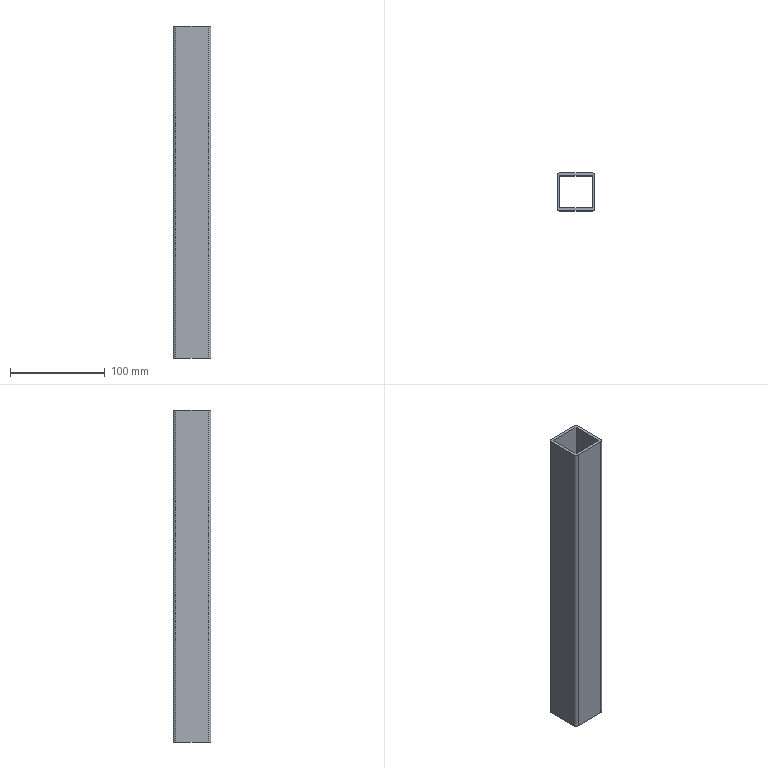Part | STEP file | X77-03114 | 1 solid | 14 faces | box 40 x 40 x 350 mm | volume 152696 mm3 | plane 10 | cylinder 4 | commonest cylinder face diameters 6 x4
STEP:
#1=CARTESIAN_POINT('',(-20.,-17.,350.));
#2=VERTEX_POINT('',#1);
#3=CARTESIAN_POINT('',(-17.,-20.,350.));
#4=VERTEX_POINT('',#3);
#5=CARTESIAN_POINT('',(-17.,-17.,350.));
#6=DIRECTION('',(0.,0.,1.));
#7=DIRECTION('',(-1.,0.,0.));
#8=AXIS2_PLACEMENT_3D('',#5,#6,#7);
#9=CIRCLE('',#8,3.);
#10=EDGE_CURVE('',#2,#4,#9,.T.);
#11=ORIENTED_EDGE('',*,*,#10,.T.);
#12=CARTESIAN_POINT('',(17.,-20.,350.));
#13=VERTEX_POINT('',#12);
#14=CARTESIAN_POINT('',(-17.,-20.,350.));
#15=DIRECTION('',(1.,0.,0.));
#16=VECTOR('',#15,1000.);
#17=LINE('',#14,#16);
#18=EDGE_CURVE('',#4,#13,#17,.T.);
#19=ORIENTED_EDGE('',*,*,#18,.T.);
#20=CARTESIAN_POINT('',(20.,-17.,350.));
#21=VERTEX_POINT('',#20);
#22=CARTESIAN_POINT('',(17.,-17.,350.));
#23=DIRECTION('',(0.,0.,1.));
#24=DIRECTION('',(-1.,0.,0.));
#25=AXIS2_PLACEMENT_3D('',#22,#23,#24);
#26=CIRCLE('',#25,3.);
#27=EDGE_CURVE('',#13,#21,#26,.T.);
#28=ORIENTED_EDGE('',*,*,#27,.T.);
#29=CARTESIAN_POINT('',(20.,17.,350.));
#30=VERTEX_POINT('',#29);
#31=CARTESIAN_POINT('',(20.,-17.,350.));
#32=DIRECTION('',(0.,1.,0.));
#33=VECTOR('',#32,1000.);
#34=LINE('',#31,#33);
#35=EDGE_CURVE('',#21,#30,#34,.T.);
#36=ORIENTED_EDGE('',*,*,#35,.T.);
#37=CARTESIAN_POINT('',(17.,20.,350.));
#38=VERTEX_POINT('',#37);
#39=CARTESIAN_POINT('',(17.,17.,350.));
#40=DIRECTION('',(0.,0.,1.));
#41=DIRECTION('',(1.,0.,0.));
#42=AXIS2_PLACEMENT_3D('',#39,#40,#41);
#43=CIRCLE('',#42,3.);
#44=EDGE_CURVE('',#30,#38,#43,.T.);
#45=ORIENTED_EDGE('',*,*,#44,.T.);
#46=CARTESIAN_POINT('',(-17.,20.,350.));
#47=VERTEX_POINT('',#46);
#48=CARTESIAN_POINT('',(-17.,20.,350.));
#49=DIRECTION('',(-1.,0.,0.));
#50=VECTOR('',#49,1000.);
#51=LINE('',#48,#50);
#52=EDGE_CURVE('',#38,#47,#51,.T.);
#53=ORIENTED_EDGE('',*,*,#52,.T.);
#54=CARTESIAN_POINT('',(-20.,17.,350.));
#55=VERTEX_POINT('',#54);
#56=CARTESIAN_POINT('',(-17.,17.,350.));
#57=DIRECTION('',(0.,0.,1.));
#58=DIRECTION('',(1.,0.,0.));
#59=AXIS2_PLACEMENT_3D('',#56,#57,#58);
#60=CIRCLE('',#59,3.);
#61=EDGE_CURVE('',#47,#55,#60,.T.);
#62=ORIENTED_EDGE('',*,*,#61,.T.);
#63=CARTESIAN_POINT('',(-20.,-17.,350.));
#64=DIRECTION('',(0.,-1.,0.));
#65=VECTOR('',#64,1000.);
#66=LINE('',#63,#65);
#67=EDGE_CURVE('',#55,#2,#66,.T.);
#68=ORIENTED_EDGE('',*,*,#67,.T.);
#69=EDGE_LOOP('',(#11,#19,#28,#36,#45,#53,#62,#68));
#70=FACE_OUTER_BOUND('',#69,.T.);
#71=CARTESIAN_POINT('',(17.,-17.,350.));
#72=VERTEX_POINT('',#71);
#73=CARTESIAN_POINT('',(17.,17.,350.));
#74=VERTEX_POINT('',#73);
#75=CARTESIAN_POINT('',(17.,-17.,350.));
#76=DIRECTION('',(0.,1.,0.));
#77=VECTOR('',#76,1000.);
#78=LINE('',#75,#77);
#79=EDGE_CURVE('',#72,#74,#78,.T.);
#80=ORIENTED_EDGE('',*,*,#79,.F.);
#81=CARTESIAN_POINT('',(-17.,-17.,350.));
#82=VERTEX_POINT('',#81);
#83=CARTESIAN_POINT('',(-17.,-17.,350.));
#84=DIRECTION('',(1.,0.,0.));
#85=VECTOR('',#84,1000.);
#86=LINE('',#83,#85);
#87=EDGE_CURVE('',#82,#72,#86,.T.);
#88=ORIENTED_EDGE('',*,*,#87,.F.);
#89=CARTESIAN_POINT('',(-17.,17.,350.));
#90=VERTEX_POINT('',#89);
#91=CARTESIAN_POINT('',(-17.,-17.,350.));
#92=DIRECTION('',(0.,-1.,0.));
#93=VECTOR('',#92,1000.);
#94=LINE('',#91,#93);
#95=EDGE_CURVE('',#90,#82,#94,.T.);
#96=ORIENTED_EDGE('',*,*,#95,.F.);
#97=CARTESIAN_POINT('',(-17.,17.,350.));
#98=DIRECTION('',(-1.,0.,0.));
#99=VECTOR('',#98,1000.);
#100=LINE('',#97,#99);
#101=EDGE_CURVE('',#74,#90,#100,.T.);
#102=ORIENTED_EDGE('',*,*,#101,.F.);
#103=EDGE_LOOP('',(#80,#88,#96,#102));
#104=FACE_BOUND('',#103,.T.);
#105=CARTESIAN_POINT('',(-17.,-17.,350.));
#106=DIRECTION('',(0.,0.,-1.));
#107=DIRECTION('',(-1.,0.,0.));
#108=AXIS2_PLACEMENT_3D('',#105,#106,#107);
#109=PLANE('',#108);
#110=ADVANCED_FACE('',(#70,#104),#109,.F.);
#111=CARTESIAN_POINT('',(-20.,-17.,0.));
#112=VERTEX_POINT('',#111);
#113=CARTESIAN_POINT('',(-17.,-20.,0.));
#114=VERTEX_POINT('',#113);
#115=CARTESIAN_POINT('',(-17.,-17.,0.));
#116=DIRECTION('',(0.,0.,1.));
#117=DIRECTION('',(-1.,0.,0.));
#118=AXIS2_PLACEMENT_3D('',#115,#116,#117);
#119=CIRCLE('',#118,3.);
#120=EDGE_CURVE('',#112,#114,#119,.T.);
#121=ORIENTED_EDGE('',*,*,#120,.F.);
#122=CARTESIAN_POINT('',(-20.,17.,0.));
#123=VERTEX_POINT('',#122);
#124=CARTESIAN_POINT('',(-20.,-17.,0.));
#125=DIRECTION('',(0.,-1.,0.));
#126=VECTOR('',#125,1000.);
#127=LINE('',#124,#126);
#128=EDGE_CURVE('',#123,#112,#127,.T.);
#129=ORIENTED_EDGE('',*,*,#128,.F.);
#130=CARTESIAN_POINT('',(-17.,20.,0.));
#131=VERTEX_POINT('',#130);
#132=CARTESIAN_POINT('',(-17.,17.,0.));
#133=DIRECTION('',(0.,0.,1.));
#134=DIRECTION('',(1.,0.,0.));
#135=AXIS2_PLACEMENT_3D('',#132,#133,#134);
#136=CIRCLE('',#135,3.);
#137=EDGE_CURVE('',#131,#123,#136,.T.);
#138=ORIENTED_EDGE('',*,*,#137,.F.);
#139=CARTESIAN_POINT('',(17.,20.,0.));
#140=VERTEX_POINT('',#139);
#141=CARTESIAN_POINT('',(-17.,20.,0.));
#142=DIRECTION('',(-1.,0.,0.));
#143=VECTOR('',#142,1000.);
#144=LINE('',#141,#143);
#145=EDGE_CURVE('',#140,#131,#144,.T.);
#146=ORIENTED_EDGE('',*,*,#145,.F.);
#147=CARTESIAN_POINT('',(20.,17.,0.));
#148=VERTEX_POINT('',#147);
#149=CARTESIAN_POINT('',(17.,17.,0.));
#150=DIRECTION('',(0.,0.,1.));
#151=DIRECTION('',(1.,0.,0.));
#152=AXIS2_PLACEMENT_3D('',#149,#150,#151);
#153=CIRCLE('',#152,3.);
#154=EDGE_CURVE('',#148,#140,#153,.T.);
#155=ORIENTED_EDGE('',*,*,#154,.F.);
#156=CARTESIAN_POINT('',(20.,-17.,0.));
#157=VERTEX_POINT('',#156);
#158=CARTESIAN_POINT('',(20.,-17.,0.));
#159=DIRECTION('',(0.,1.,0.));
#160=VECTOR('',#159,1000.);
#161=LINE('',#158,#160);
#162=EDGE_CURVE('',#157,#148,#161,.T.);
#163=ORIENTED_EDGE('',*,*,#162,.F.);
#164=CARTESIAN_POINT('',(17.,-20.,0.));
#165=VERTEX_POINT('',#164);
#166=CARTESIAN_POINT('',(17.,-17.,0.));
#167=DIRECTION('',(0.,0.,1.));
#168=DIRECTION('',(-1.,0.,0.));
#169=AXIS2_PLACEMENT_3D('',#166,#167,#168);
#170=CIRCLE('',#169,3.);
#171=EDGE_CURVE('',#165,#157,#170,.T.);
#172=ORIENTED_EDGE('',*,*,#171,.F.);
#173=CARTESIAN_POINT('',(-17.,-20.,0.));
#174=DIRECTION('',(1.,0.,0.));
#175=VECTOR('',#174,1000.);
#176=LINE('',#173,#175);
#177=EDGE_CURVE('',#114,#165,#176,.T.);
#178=ORIENTED_EDGE('',*,*,#177,.F.);
#179=EDGE_LOOP('',(#121,#129,#138,#146,#155,#163,#172,#178));
#180=FACE_OUTER_BOUND('',#179,.T.);
#181=CARTESIAN_POINT('',(-17.,-17.,0.));
#182=VERTEX_POINT('',#181);
#183=CARTESIAN_POINT('',(17.,-17.,0.));
#184=VERTEX_POINT('',#183);
#185=CARTESIAN_POINT('',(-17.,-17.,0.));
#186=DIRECTION('',(1.,0.,0.));
#187=VECTOR('',#186,1000.);
#188=LINE('',#185,#187);
#189=EDGE_CURVE('',#182,#184,#188,.T.);
#190=ORIENTED_EDGE('',*,*,#189,.T.);
#191=CARTESIAN_POINT('',(17.,17.,0.));
#192=VERTEX_POINT('',#191);
#193=CARTESIAN_POINT('',(17.,-17.,0.));
#194=DIRECTION('',(0.,1.,0.));
#195=VECTOR('',#194,1000.);
#196=LINE('',#193,#195);
#197=EDGE_CURVE('',#184,#192,#196,.T.);
#198=ORIENTED_EDGE('',*,*,#197,.T.);
#199=CARTESIAN_POINT('',(-17.,17.,0.));
#200=VERTEX_POINT('',#199);
#201=CARTESIAN_POINT('',(-17.,17.,0.));
#202=DIRECTION('',(-1.,0.,0.));
#203=VECTOR('',#202,1000.);
#204=LINE('',#201,#203);
#205=EDGE_CURVE('',#192,#200,#204,.T.);
#206=ORIENTED_EDGE('',*,*,#205,.T.);
#207=CARTESIAN_POINT('',(-17.,-17.,0.));
#208=DIRECTION('',(0.,-1.,0.));
#209=VECTOR('',#208,1000.);
#210=LINE('',#207,#209);
#211=EDGE_CURVE('',#200,#182,#210,.T.);
#212=ORIENTED_EDGE('',*,*,#211,.T.);
#213=EDGE_LOOP('',(#190,#198,#206,#212));
#214=FACE_BOUND('',#213,.T.);
#215=CARTESIAN_POINT('',(-17.,-17.,0.));
#216=DIRECTION('',(0.,0.,-1.));
#217=DIRECTION('',(-1.,0.,0.));
#218=AXIS2_PLACEMENT_3D('',#215,#216,#217);
#219=PLANE('',#218);
#220=ADVANCED_FACE('',(#180,#214),#219,.T.);
#221=ORIENTED_EDGE('',*,*,#120,.T.);
#222=CARTESIAN_POINT('',(-17.,-20.,350.));
#223=DIRECTION('',(0.,0.,-1.));
#224=VECTOR('',#223,1000.);
#225=LINE('',#222,#224);
#226=EDGE_CURVE('',#4,#114,#225,.T.);
#227=ORIENTED_EDGE('',*,*,#226,.F.);
#228=ORIENTED_EDGE('',*,*,#10,.F.);
#229=CARTESIAN_POINT('',(-20.,-17.,350.));
#230=DIRECTION('',(0.,0.,-1.));
#231=VECTOR('',#230,1000.);
#232=LINE('',#229,#231);
#233=EDGE_CURVE('',#2,#112,#232,.T.);
#234=ORIENTED_EDGE('',*,*,#233,.T.);
#235=EDGE_LOOP('',(#221,#227,#228,#234));
#236=FACE_OUTER_BOUND('',#235,.T.);
#237=CARTESIAN_POINT('',(-17.,-17.,350.));
#238=DIRECTION('',(0.,0.,-1.));
#239=DIRECTION('',(-1.,0.,0.));
#240=AXIS2_PLACEMENT_3D('',#237,#238,#239);
#241=CYLINDRICAL_SURFACE('',#240,3.);
#242=ADVANCED_FACE('',(#236),#241,.T.);
#243=ORIENTED_EDGE('',*,*,#177,.T.);
#244=CARTESIAN_POINT('',(17.,-20.,350.));
#245=DIRECTION('',(0.,0.,-1.));
#246=VECTOR('',#245,1000.);
#247=LINE('',#244,#246);
#248=EDGE_CURVE('',#13,#165,#247,.T.);
#249=ORIENTED_EDGE('',*,*,#248,.F.);
#250=ORIENTED_EDGE('',*,*,#18,.F.);
#251=ORIENTED_EDGE('',*,*,#226,.T.);
#252=EDGE_LOOP('',(#243,#249,#250,#251));
#253=FACE_OUTER_BOUND('',#252,.T.);
#254=CARTESIAN_POINT('',(-17.,-20.,350.));
#255=DIRECTION('',(0.,1.,0.));
#256=DIRECTION('',(0.,0.,1.));
#257=AXIS2_PLACEMENT_3D('',#254,#255,#256);
#258=PLANE('',#257);
#259=ADVANCED_FACE('',(#253),#258,.F.);
#260=ORIENTED_EDGE('',*,*,#171,.T.);
#261=CARTESIAN_POINT('',(20.,-17.,350.));
#262=DIRECTION('',(0.,0.,-1.));
#263=VECTOR('',#262,1000.);
#264=LINE('',#261,#263);
#265=EDGE_CURVE('',#21,#157,#264,.T.);
#266=ORIENTED_EDGE('',*,*,#265,.F.);
#267=ORIENTED_EDGE('',*,*,#27,.F.);
#268=ORIENTED_EDGE('',*,*,#248,.T.);
#269=EDGE_LOOP('',(#260,#266,#267,#268));
#270=FACE_OUTER_BOUND('',#269,.T.);
#271=CARTESIAN_POINT('',(17.,-17.,350.));
#272=DIRECTION('',(0.,0.,-1.));
#273=DIRECTION('',(-1.,0.,0.));
#274=AXIS2_PLACEMENT_3D('',#271,#272,#273);
#275=CYLINDRICAL_SURFACE('',#274,3.);
#276=ADVANCED_FACE('',(#270),#275,.T.);
#277=ORIENTED_EDGE('',*,*,#162,.T.);
#278=CARTESIAN_POINT('',(20.,17.,350.));
#279=DIRECTION('',(0.,0.,-1.));
#280=VECTOR('',#279,1000.);
#281=LINE('',#278,#280);
#282=EDGE_CURVE('',#30,#148,#281,.T.);
#283=ORIENTED_EDGE('',*,*,#282,.F.);
#284=ORIENTED_EDGE('',*,*,#35,.F.);
#285=ORIENTED_EDGE('',*,*,#265,.T.);
#286=EDGE_LOOP('',(#277,#283,#284,#285));
#287=FACE_OUTER_BOUND('',#286,.T.);
#288=CARTESIAN_POINT('',(20.,-17.,350.));
#289=DIRECTION('',(-1.,0.,0.));
#290=DIRECTION('',(0.,0.,1.));
#291=AXIS2_PLACEMENT_3D('',#288,#289,#290);
#292=PLANE('',#291);
#293=ADVANCED_FACE('',(#287),#292,.F.);
#294=ORIENTED_EDGE('',*,*,#154,.T.);
#295=CARTESIAN_POINT('',(17.,20.,350.));
#296=DIRECTION('',(0.,0.,-1.));
#297=VECTOR('',#296,1000.);
#298=LINE('',#295,#297);
#299=EDGE_CURVE('',#38,#140,#298,.T.);
#300=ORIENTED_EDGE('',*,*,#299,.F.);
#301=ORIENTED_EDGE('',*,*,#44,.F.);
#302=ORIENTED_EDGE('',*,*,#282,.T.);
#303=EDGE_LOOP('',(#294,#300,#301,#302));
#304=FACE_OUTER_BOUND('',#303,.T.);
#305=CARTESIAN_POINT('',(17.,17.,350.));
#306=DIRECTION('',(0.,0.,-1.));
#307=DIRECTION('',(-1.,0.,0.));
#308=AXIS2_PLACEMENT_3D('',#305,#306,#307);
#309=CYLINDRICAL_SURFACE('',#308,3.);
#310=ADVANCED_FACE('',(#304),#309,.T.);
#311=ORIENTED_EDGE('',*,*,#145,.T.);
#312=CARTESIAN_POINT('',(-17.,20.,350.));
#313=DIRECTION('',(0.,0.,-1.));
#314=VECTOR('',#313,1000.);
#315=LINE('',#312,#314);
#316=EDGE_CURVE('',#47,#131,#315,.T.);
#317=ORIENTED_EDGE('',*,*,#316,.F.);
#318=ORIENTED_EDGE('',*,*,#52,.F.);
#319=ORIENTED_EDGE('',*,*,#299,.T.);
#320=EDGE_LOOP('',(#311,#317,#318,#319));
#321=FACE_OUTER_BOUND('',#320,.T.);
#322=CARTESIAN_POINT('',(-17.,20.,350.));
#323=DIRECTION('',(0.,-1.,0.));
#324=DIRECTION('',(0.,0.,-1.));
#325=AXIS2_PLACEMENT_3D('',#322,#323,#324);
#326=PLANE('',#325);
#327=ADVANCED_FACE('',(#321),#326,.F.);
#328=ORIENTED_EDGE('',*,*,#137,.T.);
#329=CARTESIAN_POINT('',(-20.,17.,350.));
#330=DIRECTION('',(0.,0.,-1.));
#331=VECTOR('',#330,1000.);
#332=LINE('',#329,#331);
#333=EDGE_CURVE('',#55,#123,#332,.T.);
#334=ORIENTED_EDGE('',*,*,#333,.F.);
#335=ORIENTED_EDGE('',*,*,#61,.F.);
#336=ORIENTED_EDGE('',*,*,#316,.T.);
#337=EDGE_LOOP('',(#328,#334,#335,#336));
#338=FACE_OUTER_BOUND('',#337,.T.);
#339=CARTESIAN_POINT('',(-17.,17.,350.));
#340=DIRECTION('',(0.,0.,-1.));
#341=DIRECTION('',(-1.,0.,0.));
#342=AXIS2_PLACEMENT_3D('',#339,#340,#341);
#343=CYLINDRICAL_SURFACE('',#342,3.);
#344=ADVANCED_FACE('',(#338),#343,.T.);
#345=ORIENTED_EDGE('',*,*,#128,.T.);
#346=ORIENTED_EDGE('',*,*,#233,.F.);
#347=ORIENTED_EDGE('',*,*,#67,.F.);
#348=ORIENTED_EDGE('',*,*,#333,.T.);
#349=EDGE_LOOP('',(#345,#346,#347,#348));
#350=FACE_OUTER_BOUND('',#349,.T.);
#351=CARTESIAN_POINT('',(-20.,-17.,350.));
#352=DIRECTION('',(1.,0.,0.));
#353=DIRECTION('',(0.,0.,-1.));
#354=AXIS2_PLACEMENT_3D('',#351,#352,#353);
#355=PLANE('',#354);
#356=ADVANCED_FACE('',(#350),#355,.F.);
#357=ORIENTED_EDGE('',*,*,#197,.F.);
#358=CARTESIAN_POINT('',(17.,-17.,350.));
#359=DIRECTION('',(0.,0.,-1.));
#360=VECTOR('',#359,1000.);
#361=LINE('',#358,#360);
#362=EDGE_CURVE('',#72,#184,#361,.T.);
#363=ORIENTED_EDGE('',*,*,#362,.F.);
#364=ORIENTED_EDGE('',*,*,#79,.T.);
#365=CARTESIAN_POINT('',(17.,17.,350.));
#366=DIRECTION('',(0.,0.,-1.));
#367=VECTOR('',#366,1000.);
#368=LINE('',#365,#367);
#369=EDGE_CURVE('',#74,#192,#368,.T.);
#370=ORIENTED_EDGE('',*,*,#369,.T.);
#371=EDGE_LOOP('',(#357,#363,#364,#370));
#372=FACE_OUTER_BOUND('',#371,.T.);
#373=CARTESIAN_POINT('',(17.,-17.,350.));
#374=DIRECTION('',(-1.,0.,0.));
#375=DIRECTION('',(0.,0.,1.));
#376=AXIS2_PLACEMENT_3D('',#373,#374,#375);
#377=PLANE('',#376);
#378=ADVANCED_FACE('',(#372),#377,.T.);
#379=ORIENTED_EDGE('',*,*,#205,.F.);
#380=ORIENTED_EDGE('',*,*,#369,.F.);
#381=ORIENTED_EDGE('',*,*,#101,.T.);
#382=CARTESIAN_POINT('',(-17.,17.,350.));
#383=DIRECTION('',(0.,0.,-1.));
#384=VECTOR('',#383,1000.);
#385=LINE('',#382,#384);
#386=EDGE_CURVE('',#90,#200,#385,.T.);
#387=ORIENTED_EDGE('',*,*,#386,.T.);
#388=EDGE_LOOP('',(#379,#380,#381,#387));
#389=FACE_OUTER_BOUND('',#388,.T.);
#390=CARTESIAN_POINT('',(-17.,17.,350.));
#391=DIRECTION('',(0.,-1.,0.));
#392=DIRECTION('',(0.,0.,-1.));
#393=AXIS2_PLACEMENT_3D('',#390,#391,#392);
#394=PLANE('',#393);
#395=ADVANCED_FACE('',(#389),#394,.T.);
#396=ORIENTED_EDGE('',*,*,#211,.F.);
#397=ORIENTED_EDGE('',*,*,#386,.F.);
#398=ORIENTED_EDGE('',*,*,#95,.T.);
#399=CARTESIAN_POINT('',(-17.,-17.,350.));
#400=DIRECTION('',(0.,0.,-1.));
#401=VECTOR('',#400,1000.);
#402=LINE('',#399,#401);
#403=EDGE_CURVE('',#82,#182,#402,.T.);
#404=ORIENTED_EDGE('',*,*,#403,.T.);
#405=EDGE_LOOP('',(#396,#397,#398,#404));
#406=FACE_OUTER_BOUND('',#405,.T.);
#407=CARTESIAN_POINT('',(-17.,-17.,350.));
#408=DIRECTION('',(1.,0.,0.));
#409=DIRECTION('',(0.,0.,-1.));
#410=AXIS2_PLACEMENT_3D('',#407,#408,#409);
#411=PLANE('',#410);
#412=ADVANCED_FACE('',(#406),#411,.T.);
#413=ORIENTED_EDGE('',*,*,#189,.F.);
#414=ORIENTED_EDGE('',*,*,#403,.F.);
#415=ORIENTED_EDGE('',*,*,#87,.T.);
#416=ORIENTED_EDGE('',*,*,#362,.T.);
#417=EDGE_LOOP('',(#413,#414,#415,#416));
#418=FACE_OUTER_BOUND('',#417,.T.);
#419=CARTESIAN_POINT('',(-17.,-17.,350.));
#420=DIRECTION('',(0.,1.,0.));
#421=DIRECTION('',(0.,0.,1.));
#422=AXIS2_PLACEMENT_3D('',#419,#420,#421);
#423=PLANE('',#422);
#424=ADVANCED_FACE('',(#418),#423,.T.);
#425=CLOSED_SHELL('',(#110,#220,#242,#259,#276,#293,#310,#327,#344,#356,#378,#395,#412,#424));
#426=MANIFOLD_SOLID_BREP('',#425);
#427=CARTESIAN_POINT('',(0.,0.,0.));
#428=DIRECTION('',(0.,0.,1.));
#429=DIRECTION('',(1.,0.,0.));
#430=AXIS2_PLACEMENT_3D('',#427,#428,#429);
#431=(LENGTH_UNIT()NAMED_UNIT(*)SI_UNIT(.MILLI.,.METRE.));
#432=UNCERTAINTY_MEASURE_WITH_UNIT(LENGTH_MEASURE(0.00001),#431,'','');
#433=(NAMED_UNIT(*)PLANE_ANGLE_UNIT()SI_UNIT($,.RADIAN.));
#434=(NAMED_UNIT(*)SI_UNIT($,.STERADIAN.)SOLID_ANGLE_UNIT());
#435=(GEOMETRIC_REPRESENTATION_CONTEXT(3)GLOBAL_UNCERTAINTY_ASSIGNED_CONTEXT((#432))GLOBAL_UNIT_ASSIGNED_CONTEXT((#431,#433,#434))REPRESENTATION_CONTEXT('',''));
#436=ADVANCED_BREP_SHAPE_REPRESENTATION('',(#426,#430),#435);